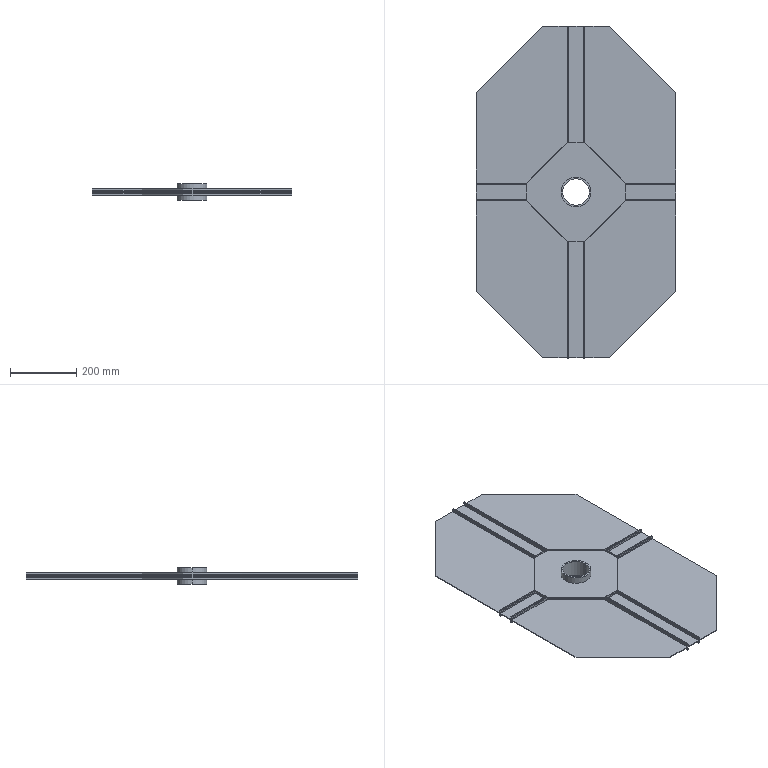Part | SolidWorks | features ICE 3, BossThin 1, Extrusion 1 | 1 solid | 148 faces | box 600 x 1000 x 50 mm | volume 1624743 mm3 | plane 142 | cylinder 6 | commonest cylinder face diameters 90 x4 80 x2